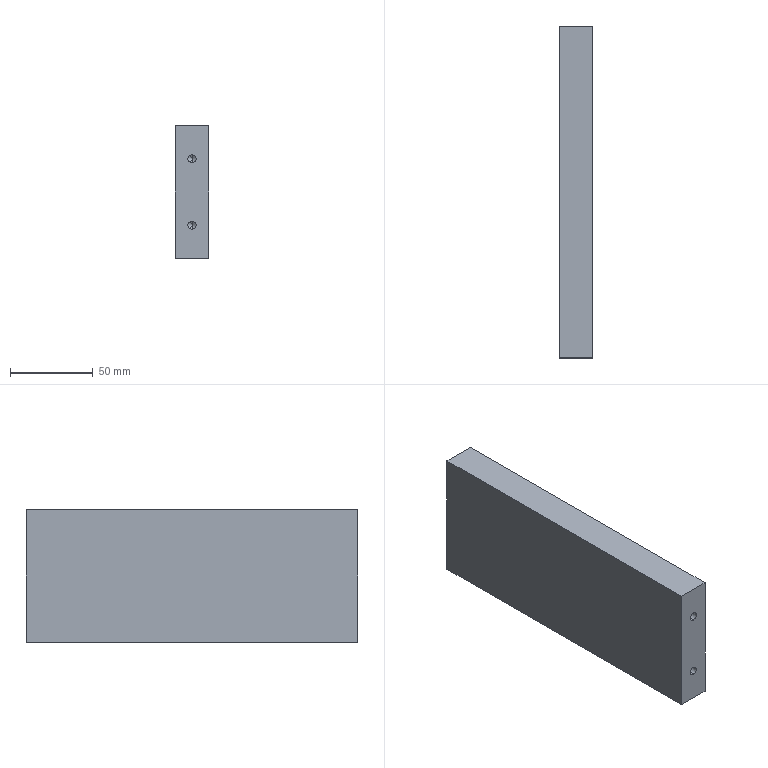Part | SolidWorks | features HoleWzd 2, Extrusion 1 | 1 solid | 22 faces | box 20 x 200 x 80 mm | volume 318272 mm3 | cylinder 8 | cone 8 | plane 6 | commonest cylinder face diameters 5 x8
STEP:
#1=CARTESIAN_POINT('',(10.,-77.,-17.5));
#2=VERTEX_POINT('',#1);
#3=CARTESIAN_POINT('',(10.,-77.,-22.5));
#4=VERTEX_POINT('',#3);
#5=CARTESIAN_POINT('',(10.,-77.,-20.));
#6=DIRECTION('',(0.,-1.,0.));
#7=DIRECTION('',(0.,0.,-1.));
#8=AXIS2_PLACEMENT_3D('',#5,#6,#7);
#9=CIRCLE('',#8,2.5);
#10=EDGE_CURVE('',#2,#4,#9,.T.);
#11=ORIENTED_EDGE('',*,*,#10,.F.);
#12=CARTESIAN_POINT('',(10.,-100.,-17.5));
#13=VERTEX_POINT('',#12);
#14=CARTESIAN_POINT('',(10.,-100.,-17.5));
#15=DIRECTION('',(0.,-1.,0.));
#16=VECTOR('',#15,1000.);
#17=LINE('',#14,#16);
#18=EDGE_CURVE('',#2,#13,#17,.T.);
#19=ORIENTED_EDGE('',*,*,#18,.T.);
#20=CARTESIAN_POINT('',(10.,-100.,-22.5));
#21=VERTEX_POINT('',#20);
#22=CARTESIAN_POINT('',(10.,-100.,-20.));
#23=DIRECTION('',(0.,-1.,0.));
#24=DIRECTION('',(0.,0.,-1.));
#25=AXIS2_PLACEMENT_3D('',#22,#23,#24);
#26=CIRCLE('',#25,2.5);
#27=EDGE_CURVE('',#13,#21,#26,.T.);
#28=ORIENTED_EDGE('',*,*,#27,.T.);
#29=CARTESIAN_POINT('',(10.,-100.,-22.5));
#30=DIRECTION('',(0.,-1.,0.));
#31=VECTOR('',#30,1000.);
#32=LINE('',#29,#31);
#33=EDGE_CURVE('',#4,#21,#32,.T.);
#34=ORIENTED_EDGE('',*,*,#33,.F.);
#35=EDGE_LOOP('',(#11,#19,#28,#34));
#36=FACE_OUTER_BOUND('',#35,.T.);
#37=CARTESIAN_POINT('',(10.,-100.,-20.));
#38=DIRECTION('',(0.,-1.,0.));
#39=DIRECTION('',(0.,0.,-1.));
#40=AXIS2_PLACEMENT_3D('',#37,#38,#39);
#41=CYLINDRICAL_SURFACE('',#40,2.5);
#42=ADVANCED_FACE('',(#36),#41,.F.);
#43=CARTESIAN_POINT('',(10.,-75.498,-20.));
#44=VERTEX_POINT('',#43);
#45=CARTESIAN_POINT('',(10.,-77.,-22.5));
#46=DIRECTION('',(0.,-0.515,-0.8572));
#47=VECTOR('',#46,1000.);
#48=LINE('',#45,#47);
#49=EDGE_CURVE('',#44,#4,#48,.T.);
#50=ORIENTED_EDGE('',*,*,#49,.F.);
#51=CARTESIAN_POINT('',(10.,-77.,-17.5));
#52=DIRECTION('',(0.,-0.515,0.8572));
#53=VECTOR('',#52,1000.);
#54=LINE('',#51,#53);
#55=EDGE_CURVE('',#44,#2,#54,.T.);
#56=ORIENTED_EDGE('',*,*,#55,.T.);
#57=ORIENTED_EDGE('',*,*,#10,.T.);
#58=EDGE_LOOP('',(#50,#56,#57));
#59=FACE_OUTER_BOUND('',#58,.T.);
#60=CARTESIAN_POINT('',(10.,-77.,-20.));
#61=DIRECTION('',(0.,-1.,0.));
#62=DIRECTION('',(0.,0.,-1.));
#63=AXIS2_PLACEMENT_3D('',#60,#61,#62);
#64=CONICAL_SURFACE('',#63,2.5,1.03);
#65=ADVANCED_FACE('',(#59),#64,.F.);
#66=CARTESIAN_POINT('',(10.,-77.,22.5));
#67=VERTEX_POINT('',#66);
#68=CARTESIAN_POINT('',(10.,-77.,17.5));
#69=VERTEX_POINT('',#68);
#70=CARTESIAN_POINT('',(10.,-77.,20.));
#71=DIRECTION('',(0.,-1.,0.));
#72=DIRECTION('',(0.,0.,-1.));
#73=AXIS2_PLACEMENT_3D('',#70,#71,#72);
#74=CIRCLE('',#73,2.5);
#75=EDGE_CURVE('',#67,#69,#74,.T.);
#76=ORIENTED_EDGE('',*,*,#75,.F.);
#77=CARTESIAN_POINT('',(10.,-100.,22.5));
#78=VERTEX_POINT('',#77);
#79=CARTESIAN_POINT('',(10.,-100.,22.5));
#80=DIRECTION('',(0.,-1.,0.));
#81=VECTOR('',#80,1000.);
#82=LINE('',#79,#81);
#83=EDGE_CURVE('',#67,#78,#82,.T.);
#84=ORIENTED_EDGE('',*,*,#83,.T.);
#85=CARTESIAN_POINT('',(10.,-100.,17.5));
#86=VERTEX_POINT('',#85);
#87=CARTESIAN_POINT('',(10.,-100.,20.));
#88=DIRECTION('',(0.,-1.,0.));
#89=DIRECTION('',(0.,0.,-1.));
#90=AXIS2_PLACEMENT_3D('',#87,#88,#89);
#91=CIRCLE('',#90,2.5);
#92=EDGE_CURVE('',#78,#86,#91,.T.);
#93=ORIENTED_EDGE('',*,*,#92,.T.);
#94=CARTESIAN_POINT('',(10.,-100.,17.5));
#95=DIRECTION('',(0.,-1.,0.));
#96=VECTOR('',#95,1000.);
#97=LINE('',#94,#96);
#98=EDGE_CURVE('',#69,#86,#97,.T.);
#99=ORIENTED_EDGE('',*,*,#98,.F.);
#100=EDGE_LOOP('',(#76,#84,#93,#99));
#101=FACE_OUTER_BOUND('',#100,.T.);
#102=CARTESIAN_POINT('',(10.,-100.,20.));
#103=DIRECTION('',(0.,-1.,0.));
#104=DIRECTION('',(0.,0.,-1.));
#105=AXIS2_PLACEMENT_3D('',#102,#103,#104);
#106=CYLINDRICAL_SURFACE('',#105,2.5);
#107=ADVANCED_FACE('',(#101),#106,.F.);
#108=CARTESIAN_POINT('',(10.,-75.498,20.));
#109=VERTEX_POINT('',#108);
#110=CARTESIAN_POINT('',(10.,-77.,17.5));
#111=DIRECTION('',(0.,-0.515,-0.8572));
#112=VECTOR('',#111,1000.);
#113=LINE('',#110,#112);
#114=EDGE_CURVE('',#109,#69,#113,.T.);
#115=ORIENTED_EDGE('',*,*,#114,.F.);
#116=CARTESIAN_POINT('',(10.,-77.,22.5));
#117=DIRECTION('',(0.,-0.515,0.8572));
#118=VECTOR('',#117,1000.);
#119=LINE('',#116,#118);
#120=EDGE_CURVE('',#109,#67,#119,.T.);
#121=ORIENTED_EDGE('',*,*,#120,.T.);
#122=ORIENTED_EDGE('',*,*,#75,.T.);
#123=EDGE_LOOP('',(#115,#121,#122));
#124=FACE_OUTER_BOUND('',#123,.T.);
#125=CARTESIAN_POINT('',(10.,-77.,20.));
#126=DIRECTION('',(0.,-1.,0.));
#127=DIRECTION('',(0.,0.,-1.));
#128=AXIS2_PLACEMENT_3D('',#125,#126,#127);
#129=CONICAL_SURFACE('',#128,2.5,1.03);
#130=ADVANCED_FACE('',(#124),#129,.F.);
#131=CARTESIAN_POINT('',(10.,80.,-15.));
#132=VERTEX_POINT('',#131);
#133=CARTESIAN_POINT('',(10.,80.,-10.));
#134=VERTEX_POINT('',#133);
#135=CARTESIAN_POINT('',(10.,80.,-12.5));
#136=DIRECTION('',(0.,1.,0.));
#137=DIRECTION('',(0.,0.,1.));
#138=AXIS2_PLACEMENT_3D('',#135,#136,#137);
#139=CIRCLE('',#138,2.5);
#140=EDGE_CURVE('',#132,#134,#139,.T.);
#141=ORIENTED_EDGE('',*,*,#140,.F.);
#142=CARTESIAN_POINT('',(10.,100.,-15.));
#143=VERTEX_POINT('',#142);
#144=CARTESIAN_POINT('',(10.,100.,-15.));
#145=DIRECTION('',(0.,1.,0.));
#146=VECTOR('',#145,1000.);
#147=LINE('',#144,#146);
#148=EDGE_CURVE('',#132,#143,#147,.T.);
#149=ORIENTED_EDGE('',*,*,#148,.T.);
#150=CARTESIAN_POINT('',(10.,100.,-10.));
#151=VERTEX_POINT('',#150);
#152=CARTESIAN_POINT('',(10.,100.,-12.5));
#153=DIRECTION('',(0.,1.,0.));
#154=DIRECTION('',(0.,0.,1.));
#155=AXIS2_PLACEMENT_3D('',#152,#153,#154);
#156=CIRCLE('',#155,2.5);
#157=EDGE_CURVE('',#143,#151,#156,.T.);
#158=ORIENTED_EDGE('',*,*,#157,.T.);
#159=CARTESIAN_POINT('',(10.,100.,-10.));
#160=DIRECTION('',(0.,1.,0.));
#161=VECTOR('',#160,1000.);
#162=LINE('',#159,#161);
#163=EDGE_CURVE('',#134,#151,#162,.T.);
#164=ORIENTED_EDGE('',*,*,#163,.F.);
#165=EDGE_LOOP('',(#141,#149,#158,#164));
#166=FACE_OUTER_BOUND('',#165,.T.);
#167=CARTESIAN_POINT('',(10.,100.,-12.5));
#168=DIRECTION('',(0.,1.,0.));
#169=DIRECTION('',(0.,0.,1.));
#170=AXIS2_PLACEMENT_3D('',#167,#168,#169);
#171=CYLINDRICAL_SURFACE('',#170,2.5);
#172=ADVANCED_FACE('',(#166),#171,.F.);
#173=CARTESIAN_POINT('',(10.,78.498,-12.5));
#174=VERTEX_POINT('',#173);
#175=CARTESIAN_POINT('',(10.,80.,-10.));
#176=DIRECTION('',(0.,0.515,0.8572));
#177=VECTOR('',#176,1000.);
#178=LINE('',#175,#177);
#179=EDGE_CURVE('',#174,#134,#178,.T.);
#180=ORIENTED_EDGE('',*,*,#179,.F.);
#181=CARTESIAN_POINT('',(10.,80.,-15.));
#182=DIRECTION('',(0.,0.515,-0.8572));
#183=VECTOR('',#182,1000.);
#184=LINE('',#181,#183);
#185=EDGE_CURVE('',#174,#132,#184,.T.);
#186=ORIENTED_EDGE('',*,*,#185,.T.);
#187=ORIENTED_EDGE('',*,*,#140,.T.);
#188=EDGE_LOOP('',(#180,#186,#187));
#189=FACE_OUTER_BOUND('',#188,.T.);
#190=CARTESIAN_POINT('',(10.,80.,-12.5));
#191=DIRECTION('',(0.,1.,0.));
#192=DIRECTION('',(0.,0.,1.));
#193=AXIS2_PLACEMENT_3D('',#190,#191,#192);
#194=CONICAL_SURFACE('',#193,2.5,1.03);
#195=ADVANCED_FACE('',(#189),#194,.F.);
#196=CARTESIAN_POINT('',(10.,80.,10.));
#197=VERTEX_POINT('',#196);
#198=CARTESIAN_POINT('',(10.,80.,15.));
#199=VERTEX_POINT('',#198);
#200=CARTESIAN_POINT('',(10.,80.,12.5));
#201=DIRECTION('',(0.,1.,0.));
#202=DIRECTION('',(0.,0.,1.));
#203=AXIS2_PLACEMENT_3D('',#200,#201,#202);
#204=CIRCLE('',#203,2.5);
#205=EDGE_CURVE('',#197,#199,#204,.T.);
#206=ORIENTED_EDGE('',*,*,#205,.F.);
#207=CARTESIAN_POINT('',(10.,100.,10.));
#208=VERTEX_POINT('',#207);
#209=CARTESIAN_POINT('',(10.,100.,10.));
#210=DIRECTION('',(0.,1.,0.));
#211=VECTOR('',#210,1000.);
#212=LINE('',#209,#211);
#213=EDGE_CURVE('',#197,#208,#212,.T.);
#214=ORIENTED_EDGE('',*,*,#213,.T.);
#215=CARTESIAN_POINT('',(10.,100.,15.));
#216=VERTEX_POINT('',#215);
#217=CARTESIAN_POINT('',(10.,100.,12.5));
#218=DIRECTION('',(0.,1.,0.));
#219=DIRECTION('',(0.,0.,1.));
#220=AXIS2_PLACEMENT_3D('',#217,#218,#219);
#221=CIRCLE('',#220,2.5);
#222=EDGE_CURVE('',#208,#216,#221,.T.);
#223=ORIENTED_EDGE('',*,*,#222,.T.);
#224=CARTESIAN_POINT('',(10.,100.,15.));
#225=DIRECTION('',(0.,1.,0.));
#226=VECTOR('',#225,1000.);
#227=LINE('',#224,#226);
#228=EDGE_CURVE('',#199,#216,#227,.T.);
#229=ORIENTED_EDGE('',*,*,#228,.F.);
#230=EDGE_LOOP('',(#206,#214,#223,#229));
#231=FACE_OUTER_BOUND('',#230,.T.);
#232=CARTESIAN_POINT('',(10.,100.,12.5));
#233=DIRECTION('',(0.,1.,0.));
#234=DIRECTION('',(0.,0.,1.));
#235=AXIS2_PLACEMENT_3D('',#232,#233,#234);
#236=CYLINDRICAL_SURFACE('',#235,2.5);
#237=ADVANCED_FACE('',(#231),#236,.F.);
#238=CARTESIAN_POINT('',(10.,78.498,12.5));
#239=VERTEX_POINT('',#238);
#240=CARTESIAN_POINT('',(10.,80.,15.));
#241=DIRECTION('',(0.,0.515,0.8572));
#242=VECTOR('',#241,1000.);
#243=LINE('',#240,#242);
#244=EDGE_CURVE('',#239,#199,#243,.T.);
#245=ORIENTED_EDGE('',*,*,#244,.F.);
#246=CARTESIAN_POINT('',(10.,80.,10.));
#247=DIRECTION('',(0.,0.515,-0.8572));
#248=VECTOR('',#247,1000.);
#249=LINE('',#246,#248);
#250=EDGE_CURVE('',#239,#197,#249,.T.);
#251=ORIENTED_EDGE('',*,*,#250,.T.);
#252=ORIENTED_EDGE('',*,*,#205,.T.);
#253=EDGE_LOOP('',(#245,#251,#252));
#254=FACE_OUTER_BOUND('',#253,.T.);
#255=CARTESIAN_POINT('',(10.,80.,12.5));
#256=DIRECTION('',(0.,1.,0.));
#257=DIRECTION('',(0.,0.,1.));
#258=AXIS2_PLACEMENT_3D('',#255,#256,#257);
#259=CONICAL_SURFACE('',#258,2.5,1.03);
#260=ADVANCED_FACE('',(#254),#259,.F.);
#261=CARTESIAN_POINT('',(0.,-100.,-40.));
#262=VERTEX_POINT('',#261);
#263=CARTESIAN_POINT('',(0.,100.,-40.));
#264=VERTEX_POINT('',#263);
#265=CARTESIAN_POINT('',(0.,100.,-40.));
#266=DIRECTION('',(0.,1.,0.));
#267=VECTOR('',#266,1000.);
#268=LINE('',#265,#267);
#269=EDGE_CURVE('',#262,#264,#268,.T.);
#270=ORIENTED_EDGE('',*,*,#269,.T.);
#271=CARTESIAN_POINT('',(20.,100.,-40.));
#272=VERTEX_POINT('',#271);
#273=CARTESIAN_POINT('',(20.,100.,-40.));
#274=DIRECTION('',(-1.,0.,0.));
#275=VECTOR('',#274,1000.);
#276=LINE('',#273,#275);
#277=EDGE_CURVE('',#272,#264,#276,.T.);
#278=ORIENTED_EDGE('',*,*,#277,.F.);
#279=CARTESIAN_POINT('',(20.,-100.,-40.));
#280=VERTEX_POINT('',#279);
#281=CARTESIAN_POINT('',(20.,100.,-40.));
#282=DIRECTION('',(0.,1.,0.));
#283=VECTOR('',#282,1000.);
#284=LINE('',#281,#283);
#285=EDGE_CURVE('',#280,#272,#284,.T.);
#286=ORIENTED_EDGE('',*,*,#285,.F.);
#287=CARTESIAN_POINT('',(20.,-100.,-40.));
#288=DIRECTION('',(-1.,0.,0.));
#289=VECTOR('',#288,1000.);
#290=LINE('',#287,#289);
#291=EDGE_CURVE('',#280,#262,#290,.T.);
#292=ORIENTED_EDGE('',*,*,#291,.T.);
#293=EDGE_LOOP('',(#270,#278,#286,#292));
#294=FACE_OUTER_BOUND('',#293,.T.);
#295=CARTESIAN_POINT('',(20.,100.,-40.));
#296=DIRECTION('',(0.,0.,1.));
#297=DIRECTION('',(0.,-1.,0.));
#298=AXIS2_PLACEMENT_3D('',#295,#296,#297);
#299=PLANE('',#298);
#300=ADVANCED_FACE('',(#294),#299,.F.);
#301=CARTESIAN_POINT('',(10.,100.,-12.5));
#302=DIRECTION('',(0.,1.,0.));
#303=DIRECTION('',(0.,0.,1.));
#304=AXIS2_PLACEMENT_3D('',#301,#302,#303);
#305=CIRCLE('',#304,2.5);
#306=EDGE_CURVE('',#151,#143,#305,.T.);
#307=ORIENTED_EDGE('',*,*,#306,.F.);
#308=ORIENTED_EDGE('',*,*,#157,.F.);
#309=EDGE_LOOP('',(#307,#308));
#310=FACE_BOUND('',#309,.T.);
#311=CARTESIAN_POINT('',(10.,100.,12.5));
#312=DIRECTION('',(0.,1.,0.));
#313=DIRECTION('',(0.,0.,1.));
#314=AXIS2_PLACEMENT_3D('',#311,#312,#313);
#315=CIRCLE('',#314,2.5);
#316=EDGE_CURVE('',#216,#208,#315,.T.);
#317=ORIENTED_EDGE('',*,*,#316,.F.);
#318=ORIENTED_EDGE('',*,*,#222,.F.);
#319=EDGE_LOOP('',(#317,#318));
#320=FACE_BOUND('',#319,.T.);
#321=CARTESIAN_POINT('',(0.,100.,40.));
#322=VERTEX_POINT('',#321);
#323=CARTESIAN_POINT('',(0.,100.,40.));
#324=DIRECTION('',(0.,0.,1.));
#325=VECTOR('',#324,1000.);
#326=LINE('',#323,#325);
#327=EDGE_CURVE('',#264,#322,#326,.T.);
#328=ORIENTED_EDGE('',*,*,#327,.T.);
#329=CARTESIAN_POINT('',(20.,100.,40.));
#330=VERTEX_POINT('',#329);
#331=CARTESIAN_POINT('',(20.,100.,40.));
#332=DIRECTION('',(-1.,0.,0.));
#333=VECTOR('',#332,1000.);
#334=LINE('',#331,#333);
#335=EDGE_CURVE('',#330,#322,#334,.T.);
#336=ORIENTED_EDGE('',*,*,#335,.F.);
#337=CARTESIAN_POINT('',(20.,100.,40.));
#338=DIRECTION('',(0.,0.,1.));
#339=VECTOR('',#338,1000.);
#340=LINE('',#337,#339);
#341=EDGE_CURVE('',#272,#330,#340,.T.);
#342=ORIENTED_EDGE('',*,*,#341,.F.);
#343=ORIENTED_EDGE('',*,*,#277,.T.);
#344=EDGE_LOOP('',(#328,#336,#342,#343));
#345=FACE_OUTER_BOUND('',#344,.T.);
#346=CARTESIAN_POINT('',(20.,100.,40.));
#347=DIRECTION('',(0.,-1.,0.));
#348=DIRECTION('',(0.,0.,-1.));
#349=AXIS2_PLACEMENT_3D('',#346,#347,#348);
#350=PLANE('',#349);
#351=ADVANCED_FACE('',(#310,#320,#345),#350,.F.);
#352=CARTESIAN_POINT('',(0.,-100.,40.));
#353=VERTEX_POINT('',#352);
#354=CARTESIAN_POINT('',(0.,100.,40.));
#355=DIRECTION('',(0.,-1.,0.));
#356=VECTOR('',#355,1000.);
#357=LINE('',#354,#356);
#358=EDGE_CURVE('',#322,#353,#357,.T.);
#359=ORIENTED_EDGE('',*,*,#358,.T.);
#360=CARTESIAN_POINT('',(20.,-100.,40.));
#361=VERTEX_POINT('',#360);
#362=CARTESIAN_POINT('',(20.,-100.,40.));
#363=DIRECTION('',(-1.,0.,0.));
#364=VECTOR('',#363,1000.);
#365=LINE('',#362,#364);
#366=EDGE_CURVE('',#361,#353,#365,.T.);
#367=ORIENTED_EDGE('',*,*,#366,.F.);
#368=CARTESIAN_POINT('',(20.,100.,40.));
#369=DIRECTION('',(0.,-1.,0.));
#370=VECTOR('',#369,1000.);
#371=LINE('',#368,#370);
#372=EDGE_CURVE('',#330,#361,#371,.T.);
#373=ORIENTED_EDGE('',*,*,#372,.F.);
#374=ORIENTED_EDGE('',*,*,#335,.T.);
#375=EDGE_LOOP('',(#359,#367,#373,#374));
#376=FACE_OUTER_BOUND('',#375,.T.);
#377=CARTESIAN_POINT('',(20.,100.,40.));
#378=DIRECTION('',(0.,0.,-1.));
#379=DIRECTION('',(0.,1.,0.));
#380=AXIS2_PLACEMENT_3D('',#377,#378,#379);
#381=PLANE('',#380);
#382=ADVANCED_FACE('',(#376),#381,.F.);
#383=CARTESIAN_POINT('',(10.,-100.,-20.));
#384=DIRECTION('',(0.,-1.,0.));
#385=DIRECTION('',(0.,0.,-1.));
#386=AXIS2_PLACEMENT_3D('',#383,#384,#385);
#387=CIRCLE('',#386,2.5);
#388=EDGE_CURVE('',#21,#13,#387,.T.);
#389=ORIENTED_EDGE('',*,*,#388,.F.);
#390=ORIENTED_EDGE('',*,*,#27,.F.);
#391=EDGE_LOOP('',(#389,#390));
#392=FACE_BOUND('',#391,.T.);
#393=CARTESIAN_POINT('',(10.,-100.,20.));
#394=DIRECTION('',(0.,-1.,0.));
#395=DIRECTION('',(0.,0.,-1.));
#396=AXIS2_PLACEMENT_3D('',#393,#394,#395);
#397=CIRCLE('',#396,2.5);
#398=EDGE_CURVE('',#86,#78,#397,.T.);
#399=ORIENTED_EDGE('',*,*,#398,.F.);
#400=ORIENTED_EDGE('',*,*,#92,.F.);
#401=EDGE_LOOP('',(#399,#400));
#402=FACE_BOUND('',#401,.T.);
#403=CARTESIAN_POINT('',(0.,-100.,40.));
#404=DIRECTION('',(0.,0.,-1.));
#405=VECTOR('',#404,1000.);
#406=LINE('',#403,#405);
#407=EDGE_CURVE('',#353,#262,#406,.T.);
#408=ORIENTED_EDGE('',*,*,#407,.T.);
#409=ORIENTED_EDGE('',*,*,#291,.F.);
#410=CARTESIAN_POINT('',(20.,-100.,40.));
#411=DIRECTION('',(0.,0.,-1.));
#412=VECTOR('',#411,1000.);
#413=LINE('',#410,#412);
#414=EDGE_CURVE('',#361,#280,#413,.T.);
#415=ORIENTED_EDGE('',*,*,#414,.F.);
#416=ORIENTED_EDGE('',*,*,#366,.T.);
#417=EDGE_LOOP('',(#408,#409,#415,#416));
#418=FACE_OUTER_BOUND('',#417,.T.);
#419=CARTESIAN_POINT('',(20.,-100.,40.));
#420=DIRECTION('',(0.,1.,0.));
#421=DIRECTION('',(0.,0.,1.));
#422=AXIS2_PLACEMENT_3D('',#419,#420,#421);
#423=PLANE('',#422);
#424=ADVANCED_FACE('',(#392,#402,#418),#423,.F.);
#425=ORIENTED_EDGE('',*,*,#285,.T.);
#426=ORIENTED_EDGE('',*,*,#341,.T.);
#427=ORIENTED_EDGE('',*,*,#372,.T.);
#428=ORIENTED_EDGE('',*,*,#414,.T.);
#429=EDGE_LOOP('',(#425,#426,#427,#428));
#430=FACE_OUTER_BOUND('',#429,.T.);
#431=CARTESIAN_POINT('',(20.,0.,0.));
#432=DIRECTION('',(1.,0.,0.));
#433=DIRECTION('',(0.,0.,-1.));
#434=AXIS2_PLACEMENT_3D('',#431,#432,#433);
#435=PLANE('',#434);
#436=ADVANCED_FACE('',(#430),#435,.T.);
#437=ORIENTED_EDGE('',*,*,#269,.F.);
#438=ORIENTED_EDGE('',*,*,#407,.F.);
#439=ORIENTED_EDGE('',*,*,#358,.F.);
#440=ORIENTED_EDGE('',*,*,#327,.F.);
#441=EDGE_LOOP('',(#437,#438,#439,#440));
#442=FACE_OUTER_BOUND('',#441,.T.);
#443=CARTESIAN_POINT('',(0.,0.,0.));
#444=DIRECTION('',(1.,0.,0.));
#445=DIRECTION('',(0.,0.,-1.));
#446=AXIS2_PLACEMENT_3D('',#443,#444,#445);
#447=PLANE('',#446);
#448=ADVANCED_FACE('',(#442),#447,.F.);
#449=ORIENTED_EDGE('',*,*,#250,.F.);
#450=ORIENTED_EDGE('',*,*,#244,.T.);
#451=CARTESIAN_POINT('',(10.,80.,12.5));
#452=DIRECTION('',(0.,1.,0.));
#453=DIRECTION('',(0.,0.,1.));
#454=AXIS2_PLACEMENT_3D('',#451,#452,#453);
#455=CIRCLE('',#454,2.5);
#456=EDGE_CURVE('',#199,#197,#455,.T.);
#457=ORIENTED_EDGE('',*,*,#456,.T.);
#458=EDGE_LOOP('',(#449,#450,#457));
#459=FACE_OUTER_BOUND('',#458,.T.);
#460=CARTESIAN_POINT('',(10.,80.,12.5));
#461=DIRECTION('',(0.,1.,0.));
#462=DIRECTION('',(0.,0.,1.));
#463=AXIS2_PLACEMENT_3D('',#460,#461,#462);
#464=CONICAL_SURFACE('',#463,2.5,1.03);
#465=ADVANCED_FACE('',(#459),#464,.F.);
#466=ORIENTED_EDGE('',*,*,#213,.F.);
#467=ORIENTED_EDGE('',*,*,#456,.F.);
#468=ORIENTED_EDGE('',*,*,#228,.T.);
#469=ORIENTED_EDGE('',*,*,#316,.T.);
#470=EDGE_LOOP('',(#466,#467,#468,#469));
#471=FACE_OUTER_BOUND('',#470,.T.);
#472=CARTESIAN_POINT('',(10.,100.,12.5));
#473=DIRECTION('',(0.,1.,0.));
#474=DIRECTION('',(0.,0.,1.));
#475=AXIS2_PLACEMENT_3D('',#472,#473,#474);
#476=CYLINDRICAL_SURFACE('',#475,2.5);
#477=ADVANCED_FACE('',(#471),#476,.F.);
#478=ORIENTED_EDGE('',*,*,#185,.F.);
#479=ORIENTED_EDGE('',*,*,#179,.T.);
#480=CARTESIAN_POINT('',(10.,80.,-12.5));
#481=DIRECTION('',(0.,1.,0.));
#482=DIRECTION('',(0.,0.,1.));
#483=AXIS2_PLACEMENT_3D('',#480,#481,#482);
#484=CIRCLE('',#483,2.5);
#485=EDGE_CURVE('',#134,#132,#484,.T.);
#486=ORIENTED_EDGE('',*,*,#485,.T.);
#487=EDGE_LOOP('',(#478,#479,#486));
#488=FACE_OUTER_BOUND('',#487,.T.);
#489=CARTESIAN_POINT('',(10.,80.,-12.5));
#490=DIRECTION('',(0.,1.,0.));
#491=DIRECTION('',(0.,0.,1.));
#492=AXIS2_PLACEMENT_3D('',#489,#490,#491);
#493=CONICAL_SURFACE('',#492,2.5,1.03);
#494=ADVANCED_FACE('',(#488),#493,.F.);
#495=ORIENTED_EDGE('',*,*,#148,.F.);
#496=ORIENTED_EDGE('',*,*,#485,.F.);
#497=ORIENTED_EDGE('',*,*,#163,.T.);
#498=ORIENTED_EDGE('',*,*,#306,.T.);
#499=EDGE_LOOP('',(#495,#496,#497,#498));
#500=FACE_OUTER_BOUND('',#499,.T.);
#501=CARTESIAN_POINT('',(10.,100.,-12.5));
#502=DIRECTION('',(0.,1.,0.));
#503=DIRECTION('',(0.,0.,1.));
#504=AXIS2_PLACEMENT_3D('',#501,#502,#503);
#505=CYLINDRICAL_SURFACE('',#504,2.5);
#506=ADVANCED_FACE('',(#500),#505,.F.);
#507=ORIENTED_EDGE('',*,*,#120,.F.);
#508=ORIENTED_EDGE('',*,*,#114,.T.);
#509=CARTESIAN_POINT('',(10.,-77.,20.));
#510=DIRECTION('',(0.,-1.,0.));
#511=DIRECTION('',(0.,0.,-1.));
#512=AXIS2_PLACEMENT_3D('',#509,#510,#511);
#513=CIRCLE('',#512,2.5);
#514=EDGE_CURVE('',#69,#67,#513,.T.);
#515=ORIENTED_EDGE('',*,*,#514,.T.);
#516=EDGE_LOOP('',(#507,#508,#515));
#517=FACE_OUTER_BOUND('',#516,.T.);
#518=CARTESIAN_POINT('',(10.,-77.,20.));
#519=DIRECTION('',(0.,-1.,0.));
#520=DIRECTION('',(0.,0.,-1.));
#521=AXIS2_PLACEMENT_3D('',#518,#519,#520);
#522=CONICAL_SURFACE('',#521,2.5,1.03);
#523=ADVANCED_FACE('',(#517),#522,.F.);
#524=ORIENTED_EDGE('',*,*,#83,.F.);
#525=ORIENTED_EDGE('',*,*,#514,.F.);
#526=ORIENTED_EDGE('',*,*,#98,.T.);
#527=ORIENTED_EDGE('',*,*,#398,.T.);
#528=EDGE_LOOP('',(#524,#525,#526,#527));
#529=FACE_OUTER_BOUND('',#528,.T.);
#530=CARTESIAN_POINT('',(10.,-100.,20.));
#531=DIRECTION('',(0.,-1.,0.));
#532=DIRECTION('',(0.,0.,-1.));
#533=AXIS2_PLACEMENT_3D('',#530,#531,#532);
#534=CYLINDRICAL_SURFACE('',#533,2.5);
#535=ADVANCED_FACE('',(#529),#534,.F.);
#536=ORIENTED_EDGE('',*,*,#55,.F.);
#537=ORIENTED_EDGE('',*,*,#49,.T.);
#538=CARTESIAN_POINT('',(10.,-77.,-20.));
#539=DIRECTION('',(0.,-1.,0.));
#540=DIRECTION('',(0.,0.,-1.));
#541=AXIS2_PLACEMENT_3D('',#538,#539,#540);
#542=CIRCLE('',#541,2.5);
#543=EDGE_CURVE('',#4,#2,#542,.T.);
#544=ORIENTED_EDGE('',*,*,#543,.T.);
#545=EDGE_LOOP('',(#536,#537,#544));
#546=FACE_OUTER_BOUND('',#545,.T.);
#547=CARTESIAN_POINT('',(10.,-77.,-20.));
#548=DIRECTION('',(0.,-1.,0.));
#549=DIRECTION('',(0.,0.,-1.));
#550=AXIS2_PLACEMENT_3D('',#547,#548,#549);
#551=CONICAL_SURFACE('',#550,2.5,1.03);
#552=ADVANCED_FACE('',(#546),#551,.F.);
#553=ORIENTED_EDGE('',*,*,#18,.F.);
#554=ORIENTED_EDGE('',*,*,#543,.F.);
#555=ORIENTED_EDGE('',*,*,#33,.T.);
#556=ORIENTED_EDGE('',*,*,#388,.T.);
#557=EDGE_LOOP('',(#553,#554,#555,#556));
#558=FACE_OUTER_BOUND('',#557,.T.);
#559=CARTESIAN_POINT('',(10.,-100.,-20.));
#560=DIRECTION('',(0.,-1.,0.));
#561=DIRECTION('',(0.,0.,-1.));
#562=AXIS2_PLACEMENT_3D('',#559,#560,#561);
#563=CYLINDRICAL_SURFACE('',#562,2.5);
#564=ADVANCED_FACE('',(#558),#563,.F.);
#565=CLOSED_SHELL('',(#42,#65,#107,#130,#172,#195,#237,#260,#300,#351,#382,#424,#436,#448,#465,#477,#494,#506,#523,#535,#552,#564));
#566=MANIFOLD_SOLID_BREP('',#565);
#567=CARTESIAN_POINT('',(0.,0.,0.));
#568=DIRECTION('',(0.,0.,1.));
#569=DIRECTION('',(1.,0.,0.));
#570=AXIS2_PLACEMENT_3D('',#567,#568,#569);
#571=(LENGTH_UNIT()NAMED_UNIT(*)SI_UNIT(.MILLI.,.METRE.));
#572=UNCERTAINTY_MEASURE_WITH_UNIT(LENGTH_MEASURE(0.00001),#571,'','');
#573=(NAMED_UNIT(*)PLANE_ANGLE_UNIT()SI_UNIT($,.RADIAN.));
#574=(NAMED_UNIT(*)SI_UNIT($,.STERADIAN.)SOLID_ANGLE_UNIT());
#575=(GEOMETRIC_REPRESENTATION_CONTEXT(3)GLOBAL_UNCERTAINTY_ASSIGNED_CONTEXT((#572))GLOBAL_UNIT_ASSIGNED_CONTEXT((#571,#573,#574))REPRESENTATION_CONTEXT('',''));
#576=ADVANCED_BREP_SHAPE_REPRESENTATION('',(#566,#570),#575);